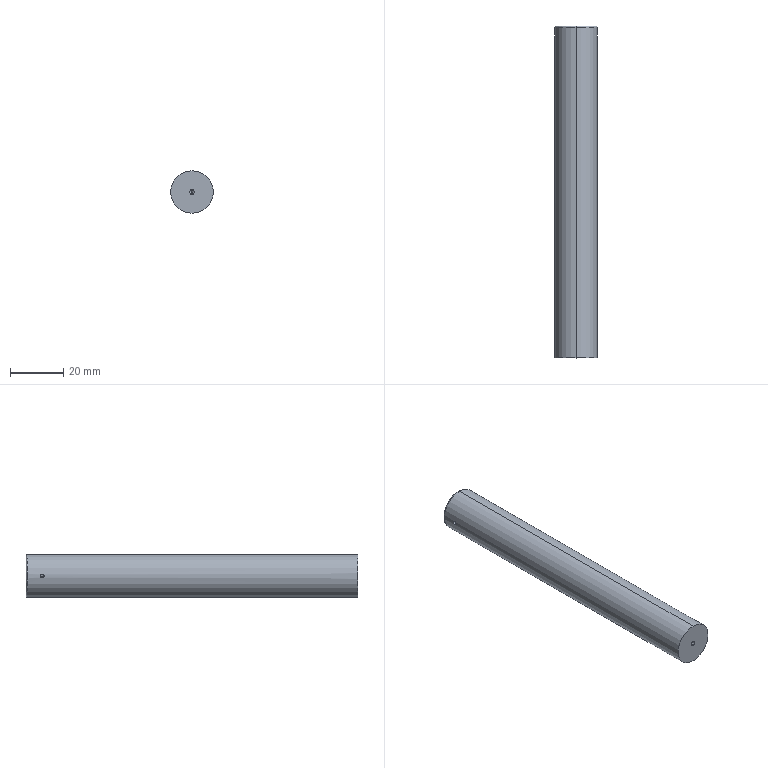Part | SolidWorks | features HoleWzd 1, RevCut 1, Revolution 1 | 1 solid | 18 faces | box 16 x 125 x 16 mm | volume 25103 mm3 | cylinder 8 | sphere 4 | cone 2 | torus 2 | plane 2 | commonest cylinder face diameters 1.4 x4 1.8 x2 16 x2
STEP:
#1=CARTESIAN_POINT('',(0.,-29.804,0.9));
#2=VERTEX_POINT('',#1);
#3=CARTESIAN_POINT('',(0.,-29.804,-0.9));
#4=VERTEX_POINT('',#3);
#5=CARTESIAN_POINT('',(0.,-29.804,0.));
#6=DIRECTION('',(0.,-1.,0.));
#7=DIRECTION('',(0.,0.,-1.));
#8=AXIS2_PLACEMENT_3D('',#5,#6,#7);
#9=CIRCLE('',#8,0.9);
#10=EDGE_CURVE('',#2,#4,#9,.T.);
#11=ORIENTED_EDGE('',*,*,#10,.F.);
#12=CARTESIAN_POINT('',(0.,-37.804,0.9));
#13=VERTEX_POINT('',#12);
#14=CARTESIAN_POINT('',(0.,-37.804,0.9));
#15=DIRECTION('',(0.,-1.,0.));
#16=VECTOR('',#15,1000.);
#17=LINE('',#14,#16);
#18=EDGE_CURVE('',#2,#13,#17,.T.);
#19=ORIENTED_EDGE('',*,*,#18,.T.);
#20=CARTESIAN_POINT('',(0.,-37.804,-0.9));
#21=VERTEX_POINT('',#20);
#22=CARTESIAN_POINT('',(0.,-37.804,0.));
#23=DIRECTION('',(0.,-1.,0.));
#24=DIRECTION('',(0.,0.,-1.));
#25=AXIS2_PLACEMENT_3D('',#22,#23,#24);
#26=CIRCLE('',#25,0.9);
#27=EDGE_CURVE('',#13,#21,#26,.T.);
#28=ORIENTED_EDGE('',*,*,#27,.T.);
#29=CARTESIAN_POINT('',(0.,-37.804,-0.9));
#30=DIRECTION('',(0.,-1.,0.));
#31=VECTOR('',#30,1000.);
#32=LINE('',#29,#31);
#33=EDGE_CURVE('',#4,#21,#32,.T.);
#34=ORIENTED_EDGE('',*,*,#33,.F.);
#35=EDGE_LOOP('',(#11,#19,#28,#34));
#36=FACE_OUTER_BOUND('',#35,.T.);
#37=CARTESIAN_POINT('',(0.,-37.804,0.));
#38=DIRECTION('',(0.,-1.,0.));
#39=DIRECTION('',(0.,0.,-1.));
#40=AXIS2_PLACEMENT_3D('',#37,#38,#39);
#41=CYLINDRICAL_SURFACE('',#40,0.9);
#42=ADVANCED_FACE('',(#36),#41,.F.);
#43=CARTESIAN_POINT('',(0.,-29.264,0.));
#44=VERTEX_POINT('',#43);
#45=CARTESIAN_POINT('',(0.,-29.804,-0.9));
#46=DIRECTION('',(0.,-0.515,-0.8572));
#47=VECTOR('',#46,1000.);
#48=LINE('',#45,#47);
#49=EDGE_CURVE('',#44,#4,#48,.T.);
#50=ORIENTED_EDGE('',*,*,#49,.F.);
#51=CARTESIAN_POINT('',(0.,-29.804,0.9));
#52=DIRECTION('',(0.,-0.515,0.8572));
#53=VECTOR('',#52,1000.);
#54=LINE('',#51,#53);
#55=EDGE_CURVE('',#44,#2,#54,.T.);
#56=ORIENTED_EDGE('',*,*,#55,.T.);
#57=ORIENTED_EDGE('',*,*,#10,.T.);
#58=EDGE_LOOP('',(#50,#56,#57));
#59=FACE_OUTER_BOUND('',#58,.T.);
#60=CARTESIAN_POINT('',(0.,-29.804,0.));
#61=DIRECTION('',(0.,-1.,0.));
#62=DIRECTION('',(0.,0.,-1.));
#63=AXIS2_PLACEMENT_3D('',#60,#61,#62);
#64=CONICAL_SURFACE('',#63,0.9,1.03);
#65=ADVANCED_FACE('',(#59),#64,.F.);
#66=CARTESIAN_POINT('',(5.8,81.114,0.));
#67=VERTEX_POINT('',#66);
#68=CARTESIAN_POINT('',(6.5,81.814,0.));
#69=VERTEX_POINT('',#68);
#70=CARTESIAN_POINT('',(6.5,81.114,0.));
#71=DIRECTION('',(0.,0.,-1.));
#72=DIRECTION('',(-1.,0.,0.));
#73=AXIS2_PLACEMENT_3D('',#70,#71,#72);
#74=CIRCLE('',#73,0.7);
#75=EDGE_CURVE('',#67,#69,#74,.T.);
#76=ORIENTED_EDGE('',*,*,#75,.F.);
#77=CARTESIAN_POINT('',(6.5,80.414,0.));
#78=VERTEX_POINT('',#77);
#79=CARTESIAN_POINT('',(6.5,81.114,0.));
#80=DIRECTION('',(0.,0.,1.));
#81=DIRECTION('',(0.,-1.,0.));
#82=AXIS2_PLACEMENT_3D('',#79,#80,#81);
#83=CIRCLE('',#82,0.7);
#84=EDGE_CURVE('',#67,#78,#83,.T.);
#85=ORIENTED_EDGE('',*,*,#84,.T.);
#86=CARTESIAN_POINT('',(6.5,81.114,-0.7));
#87=VERTEX_POINT('',#86);
#88=CARTESIAN_POINT('',(6.5,81.114,0.));
#89=DIRECTION('',(1.,0.,0.));
#90=DIRECTION('',(0.,0.,-1.));
#91=AXIS2_PLACEMENT_3D('',#88,#89,#90);
#92=CIRCLE('',#91,0.7);
#93=EDGE_CURVE('',#78,#87,#92,.T.);
#94=ORIENTED_EDGE('',*,*,#93,.T.);
#95=CARTESIAN_POINT('',(6.5,81.114,0.));
#96=DIRECTION('',(1.,0.,0.));
#97=DIRECTION('',(0.,0.,-1.));
#98=AXIS2_PLACEMENT_3D('',#95,#96,#97);
#99=CIRCLE('',#98,0.7);
#100=EDGE_CURVE('',#87,#69,#99,.T.);
#101=ORIENTED_EDGE('',*,*,#100,.T.);
#102=EDGE_LOOP('',(#76,#85,#94,#101));
#103=FACE_OUTER_BOUND('',#102,.T.);
#104=CARTESIAN_POINT('',(6.5,81.114,0.));
#105=DIRECTION('',(0.,0.,1.));
#106=DIRECTION('',(0.,1.,0.));
#107=AXIS2_PLACEMENT_3D('',#104,#105,#106);
#108=SPHERICAL_SURFACE('',#107,0.7);
#109=ADVANCED_FACE('',(#103),#108,.F.);
#110=CARTESIAN_POINT('',(6.5,81.114,0.7));
#111=VERTEX_POINT('',#110);
#112=CARTESIAN_POINT('',(6.5,81.114,0.));
#113=DIRECTION('',(1.,0.,0.));
#114=DIRECTION('',(0.,0.,-1.));
#115=AXIS2_PLACEMENT_3D('',#112,#113,#114);
#116=CIRCLE('',#115,0.7);
#117=EDGE_CURVE('',#111,#78,#116,.T.);
#118=ORIENTED_EDGE('',*,*,#117,.F.);
#119=CARTESIAN_POINT('',(7.969,81.114,0.7));
#120=VERTEX_POINT('',#119);
#121=CARTESIAN_POINT('',(8.,81.114,0.7));
#122=DIRECTION('',(1.,0.,0.));
#123=VECTOR('',#122,1000.);
#124=LINE('',#121,#123);
#125=EDGE_CURVE('',#111,#120,#124,.T.);
#126=ORIENTED_EDGE('',*,*,#125,.T.);
#127=CARTESIAN_POINT('',(7.969,81.114,-0.7));
#128=VERTEX_POINT('',#127);
#129=CARTESIAN_POINT('',(7.969,81.114,0.7));
#130=CARTESIAN_POINT('',(7.969,80.931,0.7));
#131=CARTESIAN_POINT('',(7.977,80.748,0.6243));
#132=CARTESIAN_POINT('',(7.989,80.554,0.4308));
#133=CARTESIAN_POINT('',(7.993,80.502,0.3532));
#134=CARTESIAN_POINT('',(7.998,80.432,0.1839));
#135=CARTESIAN_POINT('',(8.,80.414,0.09299));
#136=CARTESIAN_POINT('',(8.,80.414,-0.09189));
#137=CARTESIAN_POINT('',(7.998,80.432,-0.1828));
#138=CARTESIAN_POINT('',(7.993,80.502,-0.3524));
#139=CARTESIAN_POINT('',(7.989,80.554,-0.43));
#140=CARTESIAN_POINT('',(7.977,80.747,-0.6238));
#141=CARTESIAN_POINT('',(7.969,80.929,-0.7));
#142=CARTESIAN_POINT('',(7.969,81.114,-0.7));
#143=B_SPLINE_CURVE_WITH_KNOTS('',3,(#129,#130,#131,#132,#133,#134,#135,#136,#137,#138,#139,#140,#141,#142),.UNSPECIFIED.,.F.,.F.,(4,2,2,2,2,2,4),(0.00219,0.002737,0.00301,0.003284,0.003558,0.003831,0.004379),.UNSPECIFIED.);
#144=EDGE_CURVE('',#120,#128,#143,.T.);
#145=ORIENTED_EDGE('',*,*,#144,.T.);
#146=CARTESIAN_POINT('',(8.,81.114,-0.7));
#147=DIRECTION('',(1.,0.,0.));
#148=VECTOR('',#147,1000.);
#149=LINE('',#146,#148);
#150=EDGE_CURVE('',#87,#128,#149,.T.);
#151=ORIENTED_EDGE('',*,*,#150,.F.);
#152=ORIENTED_EDGE('',*,*,#93,.F.);
#153=EDGE_LOOP('',(#118,#126,#145,#151,#152));
#154=FACE_OUTER_BOUND('',#153,.T.);
#155=CARTESIAN_POINT('',(8.,81.114,0.));
#156=DIRECTION('',(1.,0.,0.));
#157=DIRECTION('',(0.,0.,-1.));
#158=AXIS2_PLACEMENT_3D('',#155,#156,#157);
#159=CYLINDRICAL_SURFACE('',#158,0.7);
#160=ADVANCED_FACE('',(#154),#159,.F.);
#161=CARTESIAN_POINT('',(-6.5,81.814,0.));
#162=VERTEX_POINT('',#161);
#163=CARTESIAN_POINT('',(-6.5,81.114,0.7));
#164=VERTEX_POINT('',#163);
#165=CARTESIAN_POINT('',(-6.5,81.114,0.));
#166=DIRECTION('',(1.,0.,0.));
#167=DIRECTION('',(0.,0.,-1.));
#168=AXIS2_PLACEMENT_3D('',#165,#166,#167);
#169=CIRCLE('',#168,0.7);
#170=EDGE_CURVE('',#162,#164,#169,.T.);
#171=ORIENTED_EDGE('',*,*,#170,.F.);
#172=CARTESIAN_POINT('',(-5.8,81.114,0.));
#173=VERTEX_POINT('',#172);
#174=CARTESIAN_POINT('',(-6.5,81.114,0.));
#175=DIRECTION('',(0.,0.,-1.));
#176=DIRECTION('',(0.,1.,0.));
#177=AXIS2_PLACEMENT_3D('',#174,#175,#176);
#178=CIRCLE('',#177,0.7);
#179=EDGE_CURVE('',#162,#173,#178,.T.);
#180=ORIENTED_EDGE('',*,*,#179,.T.);
#181=CARTESIAN_POINT('',(-6.5,80.414,0.));
#182=VERTEX_POINT('',#181);
#183=CARTESIAN_POINT('',(-6.5,81.114,0.));
#184=DIRECTION('',(0.,0.,1.));
#185=DIRECTION('',(1.,0.,0.));
#186=AXIS2_PLACEMENT_3D('',#183,#184,#185);
#187=CIRCLE('',#186,0.7);
#188=EDGE_CURVE('',#182,#173,#187,.T.);
#189=ORIENTED_EDGE('',*,*,#188,.F.);
#190=CARTESIAN_POINT('',(-6.5,81.114,0.));
#191=DIRECTION('',(1.,0.,0.));
#192=DIRECTION('',(0.,0.,-1.));
#193=AXIS2_PLACEMENT_3D('',#190,#191,#192);
#194=CIRCLE('',#193,0.7);
#195=EDGE_CURVE('',#164,#182,#194,.T.);
#196=ORIENTED_EDGE('',*,*,#195,.F.);
#197=EDGE_LOOP('',(#171,#180,#189,#196));
#198=FACE_OUTER_BOUND('',#197,.T.);
#199=CARTESIAN_POINT('',(-6.5,81.114,0.));
#200=DIRECTION('',(0.,0.,-1.));
#201=DIRECTION('',(0.,-1.,0.));
#202=AXIS2_PLACEMENT_3D('',#199,#200,#201);
#203=SPHERICAL_SURFACE('',#202,0.7);
#204=ADVANCED_FACE('',(#198),#203,.F.);
#205=CARTESIAN_POINT('',(-7.969,81.114,-0.7));
#206=VERTEX_POINT('',#205);
#207=CARTESIAN_POINT('',(-7.969,81.114,0.7));
#208=VERTEX_POINT('',#207);
#209=CARTESIAN_POINT('',(-7.969,81.114,-0.7));
#210=CARTESIAN_POINT('',(-7.969,81.021,-0.7));
#211=CARTESIAN_POINT('',(-7.971,80.93,-0.6818));
#212=CARTESIAN_POINT('',(-7.977,80.761,-0.6115));
#213=CARTESIAN_POINT('',(-7.981,80.683,-0.5594));
#214=CARTESIAN_POINT('',(-7.993,80.49,-0.3658));
#215=CARTESIAN_POINT('',(-8.,80.414,-0.183));
#216=CARTESIAN_POINT('',(-8.,80.414,0.09111));
#217=CARTESIAN_POINT('',(-7.998,80.432,0.1829));
#218=CARTESIAN_POINT('',(-7.993,80.502,0.3524));
#219=CARTESIAN_POINT('',(-7.989,80.553,0.4295));
#220=CARTESIAN_POINT('',(-7.981,80.684,0.5603));
#221=CARTESIAN_POINT('',(-7.977,80.761,0.6116));
#222=CARTESIAN_POINT('',(-7.971,80.931,0.6818));
#223=CARTESIAN_POINT('',(-7.969,81.022,0.7));
#224=CARTESIAN_POINT('',(-7.969,81.114,0.7));
#225=B_SPLINE_CURVE_WITH_KNOTS('',3,(#209,#210,#211,#212,#213,#214,#215,#216,#217,#218,#219,#220,#221,#222,#223,#224),.UNSPECIFIED.,.F.,.F.,(4,2,2,2,2,2,2,4),(0.,0.0002737,0.0005474,0.001095,0.001368,0.001642,0.001916,0.00219),.UNSPECIFIED.);
#226=EDGE_CURVE('',#206,#208,#225,.T.);
#227=ORIENTED_EDGE('',*,*,#226,.T.);
#228=CARTESIAN_POINT('',(8.,81.114,0.7));
#229=DIRECTION('',(1.,0.,0.));
#230=VECTOR('',#229,1000.);
#231=LINE('',#228,#230);
#232=EDGE_CURVE('',#208,#164,#231,.T.);
#233=ORIENTED_EDGE('',*,*,#232,.T.);
#234=ORIENTED_EDGE('',*,*,#195,.T.);
#235=CARTESIAN_POINT('',(-6.5,81.114,-0.7));
#236=VERTEX_POINT('',#235);
#237=CARTESIAN_POINT('',(-6.5,81.114,0.));
#238=DIRECTION('',(1.,0.,0.));
#239=DIRECTION('',(0.,0.,-1.));
#240=AXIS2_PLACEMENT_3D('',#237,#238,#239);
#241=CIRCLE('',#240,0.7);
#242=EDGE_CURVE('',#182,#236,#241,.T.);
#243=ORIENTED_EDGE('',*,*,#242,.T.);
#244=CARTESIAN_POINT('',(8.,81.114,-0.7));
#245=DIRECTION('',(1.,0.,0.));
#246=VECTOR('',#245,1000.);
#247=LINE('',#244,#246);
#248=EDGE_CURVE('',#206,#236,#247,.T.);
#249=ORIENTED_EDGE('',*,*,#248,.F.);
#250=EDGE_LOOP('',(#227,#233,#234,#243,#249));
#251=FACE_OUTER_BOUND('',#250,.T.);
#252=CARTESIAN_POINT('',(8.,81.114,0.));
#253=DIRECTION('',(1.,0.,0.));
#254=DIRECTION('',(0.,0.,-1.));
#255=AXIS2_PLACEMENT_3D('',#252,#253,#254);
#256=CYLINDRICAL_SURFACE('',#255,0.7);
#257=ADVANCED_FACE('',(#251),#256,.F.);
#258=CARTESIAN_POINT('',(0.,86.696,8.));
#259=VERTEX_POINT('',#258);
#260=CARTESIAN_POINT('',(0.,86.696,-8.));
#261=VERTEX_POINT('',#260);
#262=CARTESIAN_POINT('',(0.,86.696,0.));
#263=DIRECTION('',(0.,1.,0.));
#264=DIRECTION('',(0.,0.,1.));
#265=AXIS2_PLACEMENT_3D('',#262,#263,#264);
#266=CIRCLE('',#265,8.);
#267=EDGE_CURVE('',#259,#261,#266,.T.);
#268=ORIENTED_EDGE('',*,*,#267,.T.);
#269=CARTESIAN_POINT('',(0.,87.196,-7.5));
#270=VERTEX_POINT('',#269);
#271=CARTESIAN_POINT('',(0.,86.696,-7.5));
#272=DIRECTION('',(1.,0.,0.));
#273=DIRECTION('',(0.,0.,-1.));
#274=AXIS2_PLACEMENT_3D('',#271,#272,#273);
#275=CIRCLE('',#274,0.5);
#276=EDGE_CURVE('',#261,#270,#275,.T.);
#277=ORIENTED_EDGE('',*,*,#276,.T.);
#278=CARTESIAN_POINT('',(0.,87.196,7.5));
#279=VERTEX_POINT('',#278);
#280=CARTESIAN_POINT('',(0.,87.196,0.));
#281=DIRECTION('',(0.,1.,0.));
#282=DIRECTION('',(0.,0.,1.));
#283=AXIS2_PLACEMENT_3D('',#280,#281,#282);
#284=CIRCLE('',#283,7.5);
#285=EDGE_CURVE('',#279,#270,#284,.T.);
#286=ORIENTED_EDGE('',*,*,#285,.F.);
#287=CARTESIAN_POINT('',(0.,86.696,7.5));
#288=DIRECTION('',(-1.,0.,0.));
#289=DIRECTION('',(0.,0.,1.));
#290=AXIS2_PLACEMENT_3D('',#287,#288,#289);
#291=CIRCLE('',#290,0.5);
#292=EDGE_CURVE('',#259,#279,#291,.T.);
#293=ORIENTED_EDGE('',*,*,#292,.F.);
#294=EDGE_LOOP('',(#268,#277,#286,#293));
#295=FACE_OUTER_BOUND('',#294,.T.);
#296=CARTESIAN_POINT('',(0.,86.696,0.));
#297=DIRECTION('',(0.,1.,0.));
#298=DIRECTION('',(0.,0.,1.));
#299=AXIS2_PLACEMENT_3D('',#296,#297,#298);
#300=TOROIDAL_SURFACE('',#299,7.5,0.5);
#301=ADVANCED_FACE('',(#295),#300,.T.);
#302=CARTESIAN_POINT('',(7.969,81.114,-0.7));
#303=CARTESIAN_POINT('',(7.969,81.206,-0.7));
#304=CARTESIAN_POINT('',(7.971,81.297,-0.6818));
#305=CARTESIAN_POINT('',(7.977,81.467,-0.6115));
#306=CARTESIAN_POINT('',(7.981,81.544,-0.5594));
#307=CARTESIAN_POINT('',(7.993,81.738,-0.3658));
#308=CARTESIAN_POINT('',(8.,81.814,-0.183));
#309=CARTESIAN_POINT('',(8.,81.814,0.09111));
#310=CARTESIAN_POINT('',(7.998,81.796,0.1829));
#311=CARTESIAN_POINT('',(7.993,81.725,0.3524));
#312=CARTESIAN_POINT('',(7.989,81.674,0.4295));
#313=CARTESIAN_POINT('',(7.981,81.543,0.5603));
#314=CARTESIAN_POINT('',(7.977,81.466,0.6116));
#315=CARTESIAN_POINT('',(7.971,81.297,0.6818));
#316=CARTESIAN_POINT('',(7.969,81.205,0.7));
#317=CARTESIAN_POINT('',(7.969,81.114,0.7));
#318=B_SPLINE_CURVE_WITH_KNOTS('',3,(#302,#303,#304,#305,#306,#307,#308,#309,#310,#311,#312,#313,#314,#315,#316,#317),.UNSPECIFIED.,.F.,.F.,(4,2,2,2,2,2,2,4),(0.,0.0002737,0.0005474,0.001095,0.001368,0.001642,0.001916,0.00219),.UNSPECIFIED.);
#319=EDGE_CURVE('',#128,#120,#318,.T.);
#320=ORIENTED_EDGE('',*,*,#319,.F.);
#321=ORIENTED_EDGE('',*,*,#144,.F.);
#322=EDGE_LOOP('',(#320,#321));
#323=FACE_BOUND('',#322,.T.);
#324=CARTESIAN_POINT('',(0.,-37.804,8.));
#325=VERTEX_POINT('',#324);
#326=CARTESIAN_POINT('',(0.,-37.804,-8.));
#327=VERTEX_POINT('',#326);
#328=CARTESIAN_POINT('',(0.,-37.804,0.));
#329=DIRECTION('',(0.,1.,0.));
#330=DIRECTION('',(0.,0.,1.));
#331=AXIS2_PLACEMENT_3D('',#328,#329,#330);
#332=CIRCLE('',#331,8.);
#333=EDGE_CURVE('',#325,#327,#332,.T.);
#334=ORIENTED_EDGE('',*,*,#333,.T.);
#335=CARTESIAN_POINT('',(0.,38.205,-8.));
#336=DIRECTION('',(0.,1.,0.));
#337=VECTOR('',#336,1000.);
#338=LINE('',#335,#337);
#339=EDGE_CURVE('',#327,#261,#338,.T.);
#340=ORIENTED_EDGE('',*,*,#339,.T.);
#341=ORIENTED_EDGE('',*,*,#267,.F.);
#342=CARTESIAN_POINT('',(0.,38.205,8.));
#343=DIRECTION('',(0.,1.,0.));
#344=VECTOR('',#343,1000.);
#345=LINE('',#342,#344);
#346=EDGE_CURVE('',#325,#259,#345,.T.);
#347=ORIENTED_EDGE('',*,*,#346,.F.);
#348=EDGE_LOOP('',(#334,#340,#341,#347));
#349=FACE_OUTER_BOUND('',#348,.T.);
#350=CARTESIAN_POINT('',(0.,38.205,0.));
#351=DIRECTION('',(0.,1.,0.));
#352=DIRECTION('',(0.,0.,1.));
#353=AXIS2_PLACEMENT_3D('',#350,#351,#352);
#354=CYLINDRICAL_SURFACE('',#353,8.);
#355=ADVANCED_FACE('',(#323,#349),#354,.T.);
#356=CARTESIAN_POINT('',(0.,-37.804,0.));
#357=DIRECTION('',(0.,-1.,0.));
#358=DIRECTION('',(0.,0.,-1.));
#359=AXIS2_PLACEMENT_3D('',#356,#357,#358);
#360=CIRCLE('',#359,0.9);
#361=EDGE_CURVE('',#21,#13,#360,.T.);
#362=ORIENTED_EDGE('',*,*,#361,.F.);
#363=ORIENTED_EDGE('',*,*,#27,.F.);
#364=EDGE_LOOP('',(#362,#363));
#365=FACE_BOUND('',#364,.T.);
#366=ORIENTED_EDGE('',*,*,#333,.F.);
#367=CARTESIAN_POINT('',(0.,-37.804,0.));
#368=DIRECTION('',(0.,1.,0.));
#369=DIRECTION('',(0.,0.,1.));
#370=AXIS2_PLACEMENT_3D('',#367,#368,#369);
#371=CIRCLE('',#370,8.);
#372=EDGE_CURVE('',#327,#325,#371,.T.);
#373=ORIENTED_EDGE('',*,*,#372,.F.);
#374=EDGE_LOOP('',(#366,#373));
#375=FACE_OUTER_BOUND('',#374,.T.);
#376=CARTESIAN_POINT('',(0.,-37.804,0.));
#377=DIRECTION('',(0.,-1.,0.));
#378=DIRECTION('',(0.,0.,-1.));
#379=AXIS2_PLACEMENT_3D('',#376,#377,#378);
#380=PLANE('',#379);
#381=ADVANCED_FACE('',(#365,#375),#380,.T.);
#382=ORIENTED_EDGE('',*,*,#339,.F.);
#383=ORIENTED_EDGE('',*,*,#372,.T.);
#384=ORIENTED_EDGE('',*,*,#346,.T.);
#385=CARTESIAN_POINT('',(0.,86.696,0.));
#386=DIRECTION('',(0.,1.,0.));
#387=DIRECTION('',(0.,0.,1.));
#388=AXIS2_PLACEMENT_3D('',#385,#386,#387);
#389=CIRCLE('',#388,8.);
#390=EDGE_CURVE('',#261,#259,#389,.T.);
#391=ORIENTED_EDGE('',*,*,#390,.F.);
#392=EDGE_LOOP('',(#382,#383,#384,#391));
#393=FACE_OUTER_BOUND('',#392,.T.);
#394=ORIENTED_EDGE('',*,*,#226,.F.);
#395=CARTESIAN_POINT('',(-7.969,81.114,0.7));
#396=CARTESIAN_POINT('',(-7.969,81.296,0.7));
#397=CARTESIAN_POINT('',(-7.977,81.479,0.6243));
#398=CARTESIAN_POINT('',(-7.989,81.673,0.4308));
#399=CARTESIAN_POINT('',(-7.993,81.725,0.3532));
#400=CARTESIAN_POINT('',(-7.998,81.795,0.1839));
#401=CARTESIAN_POINT('',(-8.,81.814,0.09299));
#402=CARTESIAN_POINT('',(-8.,81.814,-0.09189));
#403=CARTESIAN_POINT('',(-7.998,81.796,-0.1828));
#404=CARTESIAN_POINT('',(-7.993,81.725,-0.3524));
#405=CARTESIAN_POINT('',(-7.989,81.673,-0.43));
#406=CARTESIAN_POINT('',(-7.977,81.48,-0.6238));
#407=CARTESIAN_POINT('',(-7.969,81.299,-0.7));
#408=CARTESIAN_POINT('',(-7.969,81.114,-0.7));
#409=B_SPLINE_CURVE_WITH_KNOTS('',3,(#395,#396,#397,#398,#399,#400,#401,#402,#403,#404,#405,#406,#407,#408),.UNSPECIFIED.,.F.,.F.,(4,2,2,2,2,2,4),(0.00219,0.002737,0.00301,0.003284,0.003558,0.003831,0.004379),.UNSPECIFIED.);
#410=EDGE_CURVE('',#208,#206,#409,.T.);
#411=ORIENTED_EDGE('',*,*,#410,.F.);
#412=EDGE_LOOP('',(#394,#411));
#413=FACE_BOUND('',#412,.T.);
#414=CARTESIAN_POINT('',(0.,38.205,0.));
#415=DIRECTION('',(0.,1.,0.));
#416=DIRECTION('',(0.,0.,1.));
#417=AXIS2_PLACEMENT_3D('',#414,#415,#416);
#418=CYLINDRICAL_SURFACE('',#417,8.);
#419=ADVANCED_FACE('',(#393,#413),#418,.T.);
#420=ORIENTED_EDGE('',*,*,#276,.F.);
#421=ORIENTED_EDGE('',*,*,#390,.T.);
#422=ORIENTED_EDGE('',*,*,#292,.T.);
#423=CARTESIAN_POINT('',(0.,87.196,0.));
#424=DIRECTION('',(0.,1.,0.));
#425=DIRECTION('',(0.,0.,1.));
#426=AXIS2_PLACEMENT_3D('',#423,#424,#425);
#427=CIRCLE('',#426,7.5);
#428=EDGE_CURVE('',#270,#279,#427,.T.);
#429=ORIENTED_EDGE('',*,*,#428,.F.);
#430=EDGE_LOOP('',(#420,#421,#422,#429));
#431=FACE_OUTER_BOUND('',#430,.T.);
#432=CARTESIAN_POINT('',(0.,86.696,0.));
#433=DIRECTION('',(0.,1.,0.));
#434=DIRECTION('',(0.,0.,1.));
#435=AXIS2_PLACEMENT_3D('',#432,#433,#434);
#436=TOROIDAL_SURFACE('',#435,7.5,0.5);
#437=ADVANCED_FACE('',(#431),#436,.T.);
#438=ORIENTED_EDGE('',*,*,#285,.T.);
#439=ORIENTED_EDGE('',*,*,#428,.T.);
#440=EDGE_LOOP('',(#438,#439));
#441=FACE_OUTER_BOUND('',#440,.T.);
#442=CARTESIAN_POINT('',(-7.5,87.196,0.));
#443=DIRECTION('',(0.,1.,0.));
#444=DIRECTION('',(0.,0.,1.));
#445=AXIS2_PLACEMENT_3D('',#442,#443,#444);
#446=PLANE('',#445);
#447=ADVANCED_FACE('',(#441),#446,.T.);
#448=ORIENTED_EDGE('',*,*,#232,.F.);
#449=ORIENTED_EDGE('',*,*,#410,.T.);
#450=ORIENTED_EDGE('',*,*,#248,.T.);
#451=CARTESIAN_POINT('',(-6.5,81.114,0.));
#452=DIRECTION('',(1.,0.,0.));
#453=DIRECTION('',(0.,0.,-1.));
#454=AXIS2_PLACEMENT_3D('',#451,#452,#453);
#455=CIRCLE('',#454,0.7);
#456=EDGE_CURVE('',#236,#162,#455,.T.);
#457=ORIENTED_EDGE('',*,*,#456,.T.);
#458=ORIENTED_EDGE('',*,*,#170,.T.);
#459=EDGE_LOOP('',(#448,#449,#450,#457,#458));
#460=FACE_OUTER_BOUND('',#459,.T.);
#461=CARTESIAN_POINT('',(8.,81.114,0.));
#462=DIRECTION('',(1.,0.,0.));
#463=DIRECTION('',(0.,0.,-1.));
#464=AXIS2_PLACEMENT_3D('',#461,#462,#463);
#465=CYLINDRICAL_SURFACE('',#464,0.7);
#466=ADVANCED_FACE('',(#460),#465,.F.);
#467=ORIENTED_EDGE('',*,*,#179,.F.);
#468=ORIENTED_EDGE('',*,*,#456,.F.);
#469=ORIENTED_EDGE('',*,*,#242,.F.);
#470=ORIENTED_EDGE('',*,*,#188,.T.);
#471=EDGE_LOOP('',(#467,#468,#469,#470));
#472=FACE_OUTER_BOUND('',#471,.T.);
#473=CARTESIAN_POINT('',(-6.5,81.114,0.));
#474=DIRECTION('',(0.,0.,-1.));
#475=DIRECTION('',(0.,-1.,0.));
#476=AXIS2_PLACEMENT_3D('',#473,#474,#475);
#477=SPHERICAL_SURFACE('',#476,0.7);
#478=ADVANCED_FACE('',(#472),#477,.F.);
#479=ORIENTED_EDGE('',*,*,#125,.F.);
#480=CARTESIAN_POINT('',(6.5,81.114,0.));
#481=DIRECTION('',(1.,0.,0.));
#482=DIRECTION('',(0.,0.,-1.));
#483=AXIS2_PLACEMENT_3D('',#480,#481,#482);
#484=CIRCLE('',#483,0.7);
#485=EDGE_CURVE('',#69,#111,#484,.T.);
#486=ORIENTED_EDGE('',*,*,#485,.F.);
#487=ORIENTED_EDGE('',*,*,#100,.F.);
#488=ORIENTED_EDGE('',*,*,#150,.T.);
#489=ORIENTED_EDGE('',*,*,#319,.T.);
#490=EDGE_LOOP('',(#479,#486,#487,#488,#489));
#491=FACE_OUTER_BOUND('',#490,.T.);
#492=CARTESIAN_POINT('',(8.,81.114,0.));
#493=DIRECTION('',(1.,0.,0.));
#494=DIRECTION('',(0.,0.,-1.));
#495=AXIS2_PLACEMENT_3D('',#492,#493,#494);
#496=CYLINDRICAL_SURFACE('',#495,0.7);
#497=ADVANCED_FACE('',(#491),#496,.F.);
#498=ORIENTED_EDGE('',*,*,#84,.F.);
#499=ORIENTED_EDGE('',*,*,#75,.T.);
#500=ORIENTED_EDGE('',*,*,#485,.T.);
#501=ORIENTED_EDGE('',*,*,#117,.T.);
#502=EDGE_LOOP('',(#498,#499,#500,#501));
#503=FACE_OUTER_BOUND('',#502,.T.);
#504=CARTESIAN_POINT('',(6.5,81.114,0.));
#505=DIRECTION('',(0.,0.,1.));
#506=DIRECTION('',(0.,1.,0.));
#507=AXIS2_PLACEMENT_3D('',#504,#505,#506);
#508=SPHERICAL_SURFACE('',#507,0.7);
#509=ADVANCED_FACE('',(#503),#508,.F.);
#510=ORIENTED_EDGE('',*,*,#55,.F.);
#511=ORIENTED_EDGE('',*,*,#49,.T.);
#512=CARTESIAN_POINT('',(0.,-29.804,0.));
#513=DIRECTION('',(0.,-1.,0.));
#514=DIRECTION('',(0.,0.,-1.));
#515=AXIS2_PLACEMENT_3D('',#512,#513,#514);
#516=CIRCLE('',#515,0.9);
#517=EDGE_CURVE('',#4,#2,#516,.T.);
#518=ORIENTED_EDGE('',*,*,#517,.T.);
#519=EDGE_LOOP('',(#510,#511,#518));
#520=FACE_OUTER_BOUND('',#519,.T.);
#521=CARTESIAN_POINT('',(0.,-29.804,0.));
#522=DIRECTION('',(0.,-1.,0.));
#523=DIRECTION('',(0.,0.,-1.));
#524=AXIS2_PLACEMENT_3D('',#521,#522,#523);
#525=CONICAL_SURFACE('',#524,0.9,1.03);
#526=ADVANCED_FACE('',(#520),#525,.F.);
#527=ORIENTED_EDGE('',*,*,#18,.F.);
#528=ORIENTED_EDGE('',*,*,#517,.F.);
#529=ORIENTED_EDGE('',*,*,#33,.T.);
#530=ORIENTED_EDGE('',*,*,#361,.T.);
#531=EDGE_LOOP('',(#527,#528,#529,#530));
#532=FACE_OUTER_BOUND('',#531,.T.);
#533=CARTESIAN_POINT('',(0.,-37.804,0.));
#534=DIRECTION('',(0.,-1.,0.));
#535=DIRECTION('',(0.,0.,-1.));
#536=AXIS2_PLACEMENT_3D('',#533,#534,#535);
#537=CYLINDRICAL_SURFACE('',#536,0.9);
#538=ADVANCED_FACE('',(#532),#537,.F.);
#539=CLOSED_SHELL('',(#42,#65,#109,#160,#204,#257,#301,#355,#381,#419,#437,#447,#466,#478,#497,#509,#526,#538));
#540=MANIFOLD_SOLID_BREP('',#539);
#541=CARTESIAN_POINT('',(0.,0.,0.));
#542=DIRECTION('',(0.,0.,1.));
#543=DIRECTION('',(1.,0.,0.));
#544=AXIS2_PLACEMENT_3D('',#541,#542,#543);
#545=(LENGTH_UNIT()NAMED_UNIT(*)SI_UNIT(.MILLI.,.METRE.));
#546=UNCERTAINTY_MEASURE_WITH_UNIT(LENGTH_MEASURE(0.00001),#545,'','');
#547=(NAMED_UNIT(*)PLANE_ANGLE_UNIT()SI_UNIT($,.RADIAN.));
#548=(NAMED_UNIT(*)SI_UNIT($,.STERADIAN.)SOLID_ANGLE_UNIT());
#549=(GEOMETRIC_REPRESENTATION_CONTEXT(3)GLOBAL_UNCERTAINTY_ASSIGNED_CONTEXT((#546))GLOBAL_UNIT_ASSIGNED_CONTEXT((#545,#547,#548))REPRESENTATION_CONTEXT('',''));
#550=ADVANCED_BREP_SHAPE_REPRESENTATION('',(#540,#544),#549);